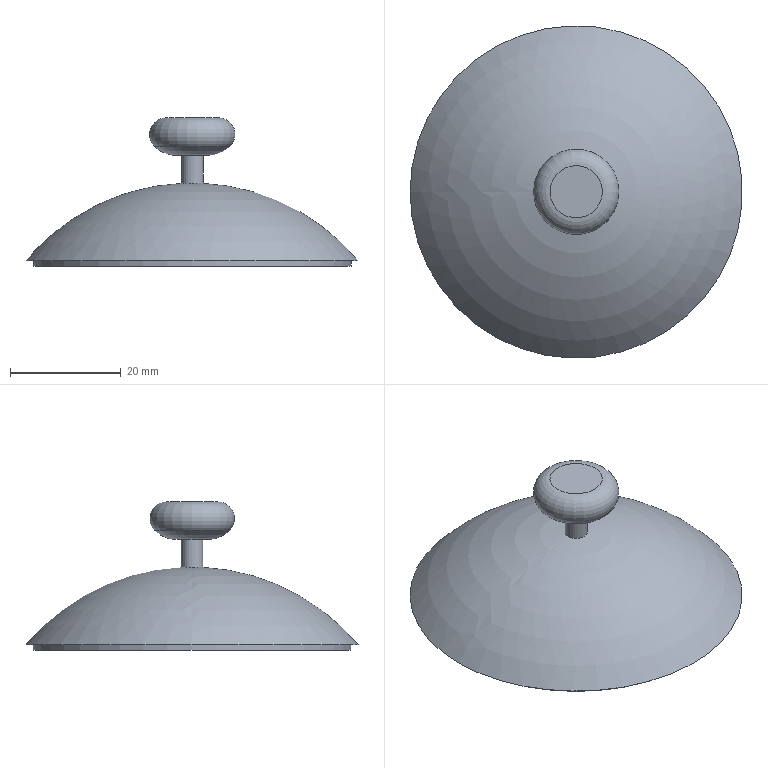Part | NX | features DATUM_CSYS 3, SKETCH 2, SWP104 2, EXTRUDE 1, SHELL 1 | 1 solid | 11 faces | box 60 x 60 x 26.776 mm | volume 4501 mm3 | plane 4 | cylinder 3 | sphere 2 | torus 2 | commonest cylinder face diameters 4 x1 56 x1 57.366 x1
STEP:
#1=CARTESIAN_POINT('',(28.683,0.,0.));
#2=VERTEX_POINT('',#1);
#3=CARTESIAN_POINT('',(0.,0.,0.));
#4=DIRECTION('',(0.,0.,1.));
#5=DIRECTION('',(1.,0.,0.));
#6=AXIS2_PLACEMENT_3D('',#3,#4,#5);
#7=CIRCLE('',#6,28.683);
#8=EDGE_CURVE('',#2,#2,#7,.F.);
#9=ORIENTED_EDGE('',*,*,#8,.F.);
#10=EDGE_LOOP('',(#9));
#11=FACE_BOUND('',#10,.T.);
#12=CARTESIAN_POINT('',(-30.,0.,0.));
#13=VERTEX_POINT('',#12);
#14=CARTESIAN_POINT('',(0.,0.,0.));
#15=DIRECTION('',(0.,0.,-1.));
#16=DIRECTION('',(-1.,0.,0.));
#17=AXIS2_PLACEMENT_3D('',#14,#15,#16);
#18=CIRCLE('',#17,30.);
#19=EDGE_CURVE('',#13,#13,#18,.T.);
#20=ORIENTED_EDGE('',*,*,#19,.T.);
#21=EDGE_LOOP('',(#20));
#22=FACE_BOUND('',#21,.T.);
#23=CARTESIAN_POINT('',(30.,0.,0.));
#24=DIRECTION('',(0.,0.,1.));
#25=DIRECTION('',(1.,0.,0.));
#26=AXIS2_PLACEMENT_3D('',#23,#24,#25);
#27=PLANE('',#26);
#28=ADVANCED_FACE('',(#11,#22),#27,.F.);
#29=CARTESIAN_POINT('',(-2.,0.,13.949));
#30=VERTEX_POINT('',#29);
#31=CARTESIAN_POINT('',(0.,0.,13.949));
#32=DIRECTION('',(0.,0.,-1.));
#33=DIRECTION('',(-1.,0.,0.));
#34=AXIS2_PLACEMENT_3D('',#31,#32,#33);
#35=CIRCLE('',#34,2.);
#36=EDGE_CURVE('',#30,#30,#35,.T.);
#37=ORIENTED_EDGE('',*,*,#36,.T.);
#38=EDGE_LOOP('',(#37));
#39=FACE_BOUND('',#38,.T.);
#40=ORIENTED_EDGE('',*,*,#19,.F.);
#41=EDGE_LOOP('',(#40));
#42=FACE_BOUND('',#41,.T.);
#43=CARTESIAN_POINT('',(0.,0.,-25.143));
#44=DIRECTION('',(0.,0.,-1.));
#45=DIRECTION('',(-1.,0.,0.));
#46=AXIS2_PLACEMENT_3D('',#43,#44,#45);
#47=SPHERICAL_SURFACE('',#46,39.143);
#48=ADVANCED_FACE('',(#39,#42),#47,.T.);
#49=CARTESIAN_POINT('',(-2.,0.,19.));
#50=VERTEX_POINT('',#49);
#51=CARTESIAN_POINT('',(0.,0.,19.));
#52=DIRECTION('',(0.,0.,-1.));
#53=DIRECTION('',(-1.,0.,0.));
#54=AXIS2_PLACEMENT_3D('',#51,#52,#53);
#55=CIRCLE('',#54,2.);
#56=EDGE_CURVE('',#50,#50,#55,.T.);
#57=ORIENTED_EDGE('',*,*,#56,.T.);
#58=EDGE_LOOP('',(#57));
#59=FACE_BOUND('',#58,.T.);
#60=ORIENTED_EDGE('',*,*,#36,.F.);
#61=EDGE_LOOP('',(#60));
#62=FACE_BOUND('',#61,.T.);
#63=CARTESIAN_POINT('',(0.,0.,14.));
#64=DIRECTION('',(0.,0.,-1.));
#65=DIRECTION('',(-1.,0.,0.));
#66=AXIS2_PLACEMENT_3D('',#63,#64,#65);
#67=CYLINDRICAL_SURFACE('',#66,2.);
#68=ADVANCED_FACE('',(#59,#62),#67,.T.);
#69=CARTESIAN_POINT('',(-6.785,0.,20.591));
#70=VERTEX_POINT('',#69);
#71=CARTESIAN_POINT('',(0.,0.,20.591));
#72=DIRECTION('',(0.,0.,-1.));
#73=DIRECTION('',(-1.,0.,0.));
#74=AXIS2_PLACEMENT_3D('',#71,#72,#73);
#75=CIRCLE('',#74,6.785);
#76=EDGE_CURVE('',#70,#70,#75,.T.);
#77=ORIENTED_EDGE('',*,*,#76,.T.);
#78=EDGE_LOOP('',(#77));
#79=FACE_BOUND('',#78,.T.);
#80=ORIENTED_EDGE('',*,*,#56,.F.);
#81=EDGE_LOOP('',(#80));
#82=FACE_BOUND('',#81,.T.);
#83=CARTESIAN_POINT('',(0.,0.,24.962));
#84=DIRECTION('',(0.,0.,-1.));
#85=DIRECTION('',(-1.,0.,0.));
#86=AXIS2_PLACEMENT_3D('',#83,#84,#85);
#87=DEGENERATE_TOROIDAL_SURFACE('',#86,2.674,6.,.T.);
#88=ADVANCED_FACE('',(#79,#82),#87,.T.);
#89=CARTESIAN_POINT('',(-4.729,0.,25.776));
#90=VERTEX_POINT('',#89);
#91=CARTESIAN_POINT('',(0.,0.,25.776));
#92=DIRECTION('',(0.,0.,-1.));
#93=DIRECTION('',(-1.,0.,0.));
#94=AXIS2_PLACEMENT_3D('',#91,#92,#93);
#95=CIRCLE('',#94,4.729);
#96=EDGE_CURVE('',#90,#90,#95,.T.);
#97=ORIENTED_EDGE('',*,*,#96,.T.);
#98=EDGE_LOOP('',(#97));
#99=FACE_BOUND('',#98,.T.);
#100=ORIENTED_EDGE('',*,*,#76,.F.);
#101=EDGE_LOOP('',(#100));
#102=FACE_BOUND('',#101,.T.);
#103=CARTESIAN_POINT('',(0.,0.,22.776));
#104=DIRECTION('',(0.,0.,-1.));
#105=DIRECTION('',(-1.,0.,0.));
#106=AXIS2_PLACEMENT_3D('',#103,#104,#105);
#107=TOROIDAL_SURFACE('',#106,4.729,3.);
#108=ADVANCED_FACE('',(#99,#102),#107,.T.);
#109=ORIENTED_EDGE('',*,*,#96,.F.);
#110=EDGE_LOOP('',(#109));
#111=FACE_BOUND('',#110,.T.);
#112=CARTESIAN_POINT('',(4.729,0.,25.776));
#113=DIRECTION('',(0.,0.,1.));
#114=DIRECTION('',(1.,0.,0.));
#115=AXIS2_PLACEMENT_3D('',#112,#113,#114);
#116=PLANE('',#115);
#117=ADVANCED_FACE('',(#111),#116,.T.);
#118=CARTESIAN_POINT('',(28.,0.,0.2));
#119=VERTEX_POINT('',#118);
#120=CARTESIAN_POINT('',(0.,0.,0.2));
#121=DIRECTION('',(0.,0.,-1.));
#122=DIRECTION('',(1.,0.,0.));
#123=AXIS2_PLACEMENT_3D('',#120,#121,#122);
#124=CIRCLE('',#123,28.);
#125=EDGE_CURVE('',#119,#119,#124,.F.);
#126=ORIENTED_EDGE('',*,*,#125,.F.);
#127=EDGE_LOOP('',(#126));
#128=FACE_BOUND('',#127,.T.);
#129=CARTESIAN_POINT('',(-28.506,0.,0.2));
#130=VERTEX_POINT('',#129);
#131=CARTESIAN_POINT('',(0.,0.,0.2));
#132=DIRECTION('',(0.,0.,-1.));
#133=DIRECTION('',(-1.,0.,0.));
#134=AXIS2_PLACEMENT_3D('',#131,#132,#133);
#135=CIRCLE('',#134,28.506);
#136=EDGE_CURVE('',#130,#130,#135,.T.);
#137=ORIENTED_EDGE('',*,*,#136,.F.);
#138=EDGE_LOOP('',(#137));
#139=FACE_BOUND('',#138,.T.);
#140=CARTESIAN_POINT('',(0.,0.,0.2));
#141=DIRECTION('',(0.,0.,-1.));
#142=DIRECTION('',(-1.,0.,0.));
#143=AXIS2_PLACEMENT_3D('',#140,#141,#142);
#144=PLANE('',#143);
#145=ADVANCED_FACE('',(#128,#139),#144,.F.);
#146=ORIENTED_EDGE('',*,*,#8,.T.);
#147=EDGE_LOOP('',(#146));
#148=FACE_BOUND('',#147,.T.);
#149=CARTESIAN_POINT('',(28.683,0.,-1.));
#150=VERTEX_POINT('',#149);
#151=CARTESIAN_POINT('',(0.,0.,-1.));
#152=DIRECTION('',(0.,0.,-1.));
#153=DIRECTION('',(1.,0.,0.));
#154=AXIS2_PLACEMENT_3D('',#151,#152,#153);
#155=CIRCLE('',#154,28.683);
#156=EDGE_CURVE('',#150,#150,#155,.F.);
#157=ORIENTED_EDGE('',*,*,#156,.T.);
#158=EDGE_LOOP('',(#157));
#159=FACE_BOUND('',#158,.T.);
#160=CARTESIAN_POINT('',(0.,0.,-1.));
#161=DIRECTION('',(0.,0.,1.));
#162=DIRECTION('',(1.,0.,0.));
#163=AXIS2_PLACEMENT_3D('',#160,#161,#162);
#164=CYLINDRICAL_SURFACE('',#163,28.683);
#165=ADVANCED_FACE('',(#148,#159),#164,.T.);
#166=CARTESIAN_POINT('',(28.,0.,-1.));
#167=VERTEX_POINT('',#166);
#168=CARTESIAN_POINT('',(0.,0.,-1.));
#169=DIRECTION('',(0.,0.,-1.));
#170=DIRECTION('',(1.,0.,0.));
#171=AXIS2_PLACEMENT_3D('',#168,#169,#170);
#172=CIRCLE('',#171,28.);
#173=EDGE_CURVE('',#167,#167,#172,.F.);
#174=ORIENTED_EDGE('',*,*,#173,.F.);
#175=EDGE_LOOP('',(#174));
#176=FACE_BOUND('',#175,.T.);
#177=ORIENTED_EDGE('',*,*,#125,.T.);
#178=EDGE_LOOP('',(#177));
#179=FACE_BOUND('',#178,.T.);
#180=CARTESIAN_POINT('',(0.,0.,-1.));
#181=DIRECTION('',(0.,0.,1.));
#182=DIRECTION('',(1.,0.,0.));
#183=AXIS2_PLACEMENT_3D('',#180,#181,#182);
#184=CYLINDRICAL_SURFACE('',#183,28.);
#185=ADVANCED_FACE('',(#176,#179),#184,.F.);
#186=ORIENTED_EDGE('',*,*,#156,.F.);
#187=EDGE_LOOP('',(#186));
#188=FACE_BOUND('',#187,.T.);
#189=ORIENTED_EDGE('',*,*,#173,.T.);
#190=EDGE_LOOP('',(#189));
#191=FACE_BOUND('',#190,.T.);
#192=CARTESIAN_POINT('',(0.,0.,-1.));
#193=DIRECTION('',(0.,0.,-1.));
#194=DIRECTION('',(-1.,0.,0.));
#195=AXIS2_PLACEMENT_3D('',#192,#193,#194);
#196=PLANE('',#195);
#197=ADVANCED_FACE('',(#188,#191),#196,.T.);
#198=ORIENTED_EDGE('',*,*,#136,.T.);
#199=EDGE_LOOP('',(#198));
#200=FACE_BOUND('',#199,.T.);
#201=CARTESIAN_POINT('',(0.,0.,-25.143));
#202=DIRECTION('',(0.,0.,-1.));
#203=DIRECTION('',(-1.,0.,0.));
#204=AXIS2_PLACEMENT_3D('',#201,#202,#203);
#205=SPHERICAL_SURFACE('',#204,38.143);
#206=ADVANCED_FACE('',(#200),#205,.F.);
#207=CLOSED_SHELL('',(#28,#48,#68,#88,#108,#117,#145,#165,#185,#197,#206));
#208=MANIFOLD_SOLID_BREP('',#207);
#209=(LENGTH_UNIT()NAMED_UNIT(*)SI_UNIT(.MILLI.,.METRE.));
#210=UNCERTAINTY_MEASURE_WITH_UNIT(LENGTH_MEASURE(0.00001),#209,'','');
#211=(NAMED_UNIT(*)PLANE_ANGLE_UNIT()SI_UNIT($,.RADIAN.));
#212=(NAMED_UNIT(*)SI_UNIT($,.STERADIAN.)SOLID_ANGLE_UNIT());
#213=(GEOMETRIC_REPRESENTATION_CONTEXT(3)GLOBAL_UNCERTAINTY_ASSIGNED_CONTEXT((#210))GLOBAL_UNIT_ASSIGNED_CONTEXT((#209,#211,#212))REPRESENTATION_CONTEXT('',''));
#214=ADVANCED_BREP_SHAPE_REPRESENTATION('',(#208),#213);